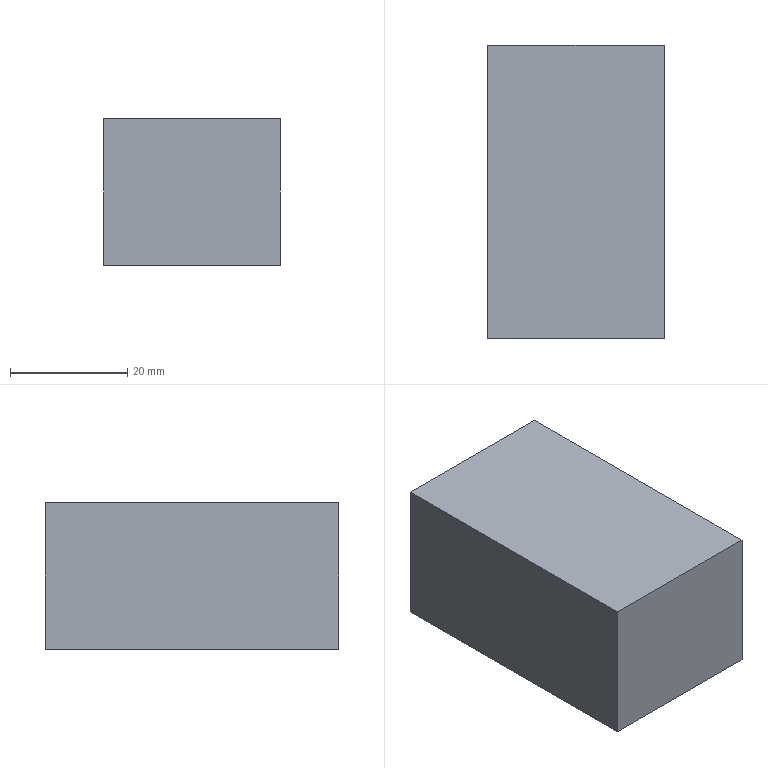Part | SolidWorks | features Extrusion 1 | 1 solid | 6 faces | box 30 x 50 x 25 mm | volume 37500 mm3 | plane 6
STEP:
#1=CARTESIAN_POINT('',(0.,50.,0.));
#2=VERTEX_POINT('',#1);
#3=CARTESIAN_POINT('',(0.,0.,0.));
#4=VERTEX_POINT('',#3);
#5=CARTESIAN_POINT('',(0.,0.,0.));
#6=DIRECTION('',(0.,-1.,0.));
#7=VECTOR('',#6,1000.);
#8=LINE('',#5,#7);
#9=EDGE_CURVE('',#2,#4,#8,.T.);
#10=ORIENTED_EDGE('',*,*,#9,.T.);
#11=CARTESIAN_POINT('',(0.,0.,25.));
#12=VERTEX_POINT('',#11);
#13=CARTESIAN_POINT('',(0.,0.,25.));
#14=DIRECTION('',(0.,0.,-1.));
#15=VECTOR('',#14,1000.);
#16=LINE('',#13,#15);
#17=EDGE_CURVE('',#12,#4,#16,.T.);
#18=ORIENTED_EDGE('',*,*,#17,.F.);
#19=CARTESIAN_POINT('',(0.,50.,25.));
#20=VERTEX_POINT('',#19);
#21=CARTESIAN_POINT('',(0.,0.,25.));
#22=DIRECTION('',(0.,-1.,0.));
#23=VECTOR('',#22,1000.);
#24=LINE('',#21,#23);
#25=EDGE_CURVE('',#20,#12,#24,.T.);
#26=ORIENTED_EDGE('',*,*,#25,.F.);
#27=CARTESIAN_POINT('',(0.,50.,25.));
#28=DIRECTION('',(0.,0.,-1.));
#29=VECTOR('',#28,1000.);
#30=LINE('',#27,#29);
#31=EDGE_CURVE('',#20,#2,#30,.T.);
#32=ORIENTED_EDGE('',*,*,#31,.T.);
#33=EDGE_LOOP('',(#10,#18,#26,#32));
#34=FACE_OUTER_BOUND('',#33,.T.);
#35=CARTESIAN_POINT('',(0.,0.,25.));
#36=DIRECTION('',(1.,0.,0.));
#37=DIRECTION('',(0.,0.,-1.));
#38=AXIS2_PLACEMENT_3D('',#35,#36,#37);
#39=PLANE('',#38);
#40=ADVANCED_FACE('',(#34),#39,.F.);
#41=CARTESIAN_POINT('',(30.,0.,0.));
#42=VERTEX_POINT('',#41);
#43=CARTESIAN_POINT('',(0.,0.,0.));
#44=DIRECTION('',(1.,0.,0.));
#45=VECTOR('',#44,1000.);
#46=LINE('',#43,#45);
#47=EDGE_CURVE('',#4,#42,#46,.T.);
#48=ORIENTED_EDGE('',*,*,#47,.T.);
#49=CARTESIAN_POINT('',(30.,0.,25.));
#50=VERTEX_POINT('',#49);
#51=CARTESIAN_POINT('',(30.,0.,25.));
#52=DIRECTION('',(0.,0.,-1.));
#53=VECTOR('',#52,1000.);
#54=LINE('',#51,#53);
#55=EDGE_CURVE('',#50,#42,#54,.T.);
#56=ORIENTED_EDGE('',*,*,#55,.F.);
#57=CARTESIAN_POINT('',(0.,0.,25.));
#58=DIRECTION('',(1.,0.,0.));
#59=VECTOR('',#58,1000.);
#60=LINE('',#57,#59);
#61=EDGE_CURVE('',#12,#50,#60,.T.);
#62=ORIENTED_EDGE('',*,*,#61,.F.);
#63=ORIENTED_EDGE('',*,*,#17,.T.);
#64=EDGE_LOOP('',(#48,#56,#62,#63));
#65=FACE_OUTER_BOUND('',#64,.T.);
#66=CARTESIAN_POINT('',(0.,0.,25.));
#67=DIRECTION('',(0.,1.,0.));
#68=DIRECTION('',(0.,0.,1.));
#69=AXIS2_PLACEMENT_3D('',#66,#67,#68);
#70=PLANE('',#69);
#71=ADVANCED_FACE('',(#65),#70,.F.);
#72=CARTESIAN_POINT('',(30.,50.,0.));
#73=VERTEX_POINT('',#72);
#74=CARTESIAN_POINT('',(30.,0.,0.));
#75=DIRECTION('',(0.,1.,0.));
#76=VECTOR('',#75,1000.);
#77=LINE('',#74,#76);
#78=EDGE_CURVE('',#42,#73,#77,.T.);
#79=ORIENTED_EDGE('',*,*,#78,.T.);
#80=CARTESIAN_POINT('',(30.,50.,25.));
#81=VERTEX_POINT('',#80);
#82=CARTESIAN_POINT('',(30.,50.,25.));
#83=DIRECTION('',(0.,0.,-1.));
#84=VECTOR('',#83,1000.);
#85=LINE('',#82,#84);
#86=EDGE_CURVE('',#81,#73,#85,.T.);
#87=ORIENTED_EDGE('',*,*,#86,.F.);
#88=CARTESIAN_POINT('',(30.,0.,25.));
#89=DIRECTION('',(0.,1.,0.));
#90=VECTOR('',#89,1000.);
#91=LINE('',#88,#90);
#92=EDGE_CURVE('',#50,#81,#91,.T.);
#93=ORIENTED_EDGE('',*,*,#92,.F.);
#94=ORIENTED_EDGE('',*,*,#55,.T.);
#95=EDGE_LOOP('',(#79,#87,#93,#94));
#96=FACE_OUTER_BOUND('',#95,.T.);
#97=CARTESIAN_POINT('',(30.,0.,25.));
#98=DIRECTION('',(-1.,0.,0.));
#99=DIRECTION('',(0.,-1.,0.));
#100=AXIS2_PLACEMENT_3D('',#97,#98,#99);
#101=PLANE('',#100);
#102=ADVANCED_FACE('',(#96),#101,.F.);
#103=CARTESIAN_POINT('',(0.,50.,0.));
#104=DIRECTION('',(-1.,0.,0.));
#105=VECTOR('',#104,1000.);
#106=LINE('',#103,#105);
#107=EDGE_CURVE('',#73,#2,#106,.T.);
#108=ORIENTED_EDGE('',*,*,#107,.T.);
#109=ORIENTED_EDGE('',*,*,#31,.F.);
#110=CARTESIAN_POINT('',(0.,50.,25.));
#111=DIRECTION('',(-1.,0.,0.));
#112=VECTOR('',#111,1000.);
#113=LINE('',#110,#112);
#114=EDGE_CURVE('',#81,#20,#113,.T.);
#115=ORIENTED_EDGE('',*,*,#114,.F.);
#116=ORIENTED_EDGE('',*,*,#86,.T.);
#117=EDGE_LOOP('',(#108,#109,#115,#116));
#118=FACE_OUTER_BOUND('',#117,.T.);
#119=CARTESIAN_POINT('',(0.,50.,25.));
#120=DIRECTION('',(0.,-1.,0.));
#121=DIRECTION('',(0.,0.,-1.));
#122=AXIS2_PLACEMENT_3D('',#119,#120,#121);
#123=PLANE('',#122);
#124=ADVANCED_FACE('',(#118),#123,.F.);
#125=ORIENTED_EDGE('',*,*,#25,.T.);
#126=ORIENTED_EDGE('',*,*,#61,.T.);
#127=ORIENTED_EDGE('',*,*,#92,.T.);
#128=ORIENTED_EDGE('',*,*,#114,.T.);
#129=EDGE_LOOP('',(#125,#126,#127,#128));
#130=FACE_OUTER_BOUND('',#129,.T.);
#131=CARTESIAN_POINT('',(0.,0.,25.));
#132=DIRECTION('',(0.,0.,-1.));
#133=DIRECTION('',(-1.,0.,0.));
#134=AXIS2_PLACEMENT_3D('',#131,#132,#133);
#135=PLANE('',#134);
#136=ADVANCED_FACE('',(#130),#135,.F.);
#137=ORIENTED_EDGE('',*,*,#9,.F.);
#138=ORIENTED_EDGE('',*,*,#107,.F.);
#139=ORIENTED_EDGE('',*,*,#78,.F.);
#140=ORIENTED_EDGE('',*,*,#47,.F.);
#141=EDGE_LOOP('',(#137,#138,#139,#140));
#142=FACE_OUTER_BOUND('',#141,.T.);
#143=CARTESIAN_POINT('',(0.,0.,0.));
#144=DIRECTION('',(0.,0.,-1.));
#145=DIRECTION('',(-1.,0.,0.));
#146=AXIS2_PLACEMENT_3D('',#143,#144,#145);
#147=PLANE('',#146);
#148=ADVANCED_FACE('',(#142),#147,.T.);
#149=CLOSED_SHELL('',(#40,#71,#102,#124,#136,#148));
#150=MANIFOLD_SOLID_BREP('',#149);
#151=CARTESIAN_POINT('',(0.,0.,0.));
#152=DIRECTION('',(0.,0.,1.));
#153=DIRECTION('',(1.,0.,0.));
#154=AXIS2_PLACEMENT_3D('',#151,#152,#153);
#155=(LENGTH_UNIT()NAMED_UNIT(*)SI_UNIT(.MILLI.,.METRE.));
#156=UNCERTAINTY_MEASURE_WITH_UNIT(LENGTH_MEASURE(0.00001),#155,'','');
#157=(NAMED_UNIT(*)PLANE_ANGLE_UNIT()SI_UNIT($,.RADIAN.));
#158=(NAMED_UNIT(*)SI_UNIT($,.STERADIAN.)SOLID_ANGLE_UNIT());
#159=(GEOMETRIC_REPRESENTATION_CONTEXT(3)GLOBAL_UNCERTAINTY_ASSIGNED_CONTEXT((#156))GLOBAL_UNIT_ASSIGNED_CONTEXT((#155,#157,#158))REPRESENTATION_CONTEXT('',''));
#160=ADVANCED_BREP_SHAPE_REPRESENTATION('',(#150,#154),#159);